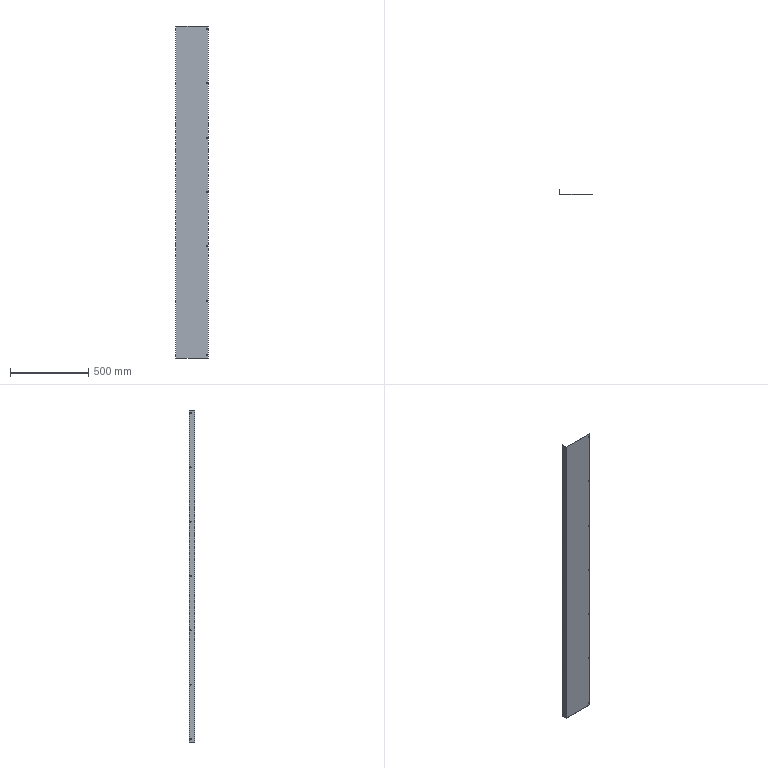Part | SolidWorks | features ICE 2, FlatPattern 1, SMBaseFlange 1, SheetMetal 1 | 1 solid | 70 faces | box 209 x 34 x 2116 mm | volume 510788 mm3 | plane 40 | cylinder 30 | commonest cylinder face diameters 6 x28 0.4 x1 2.4 x1